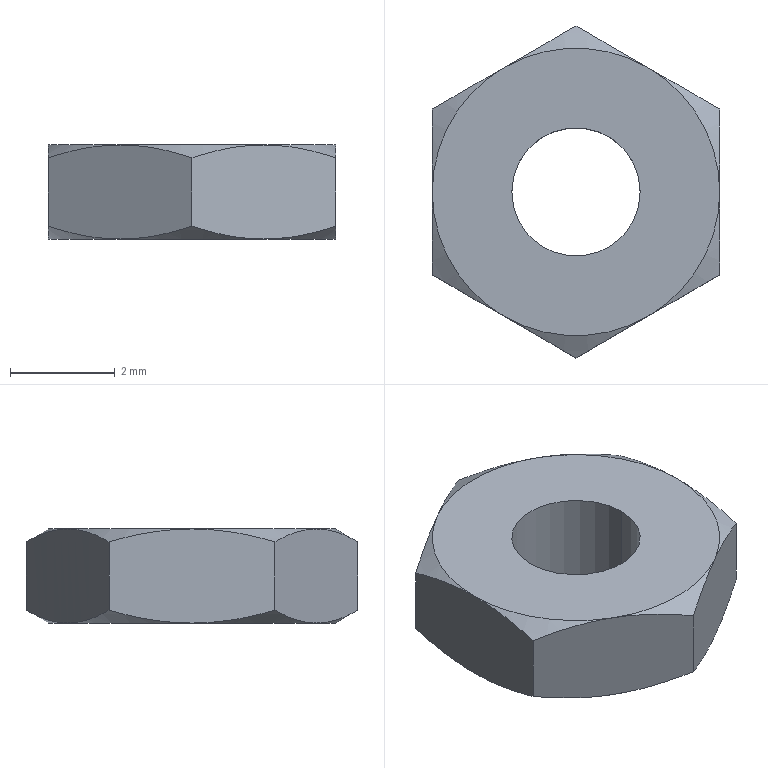Part | SolidWorks | features MBimport 1 | 1 solid | 22 faces | box 5.5 x 6.351 x 1.8 mm | volume 38.249 mm3 | cone 12 | plane 8 | cylinder 2 | commonest cylinder face diameters 2.459 x2
STEP:
#1=CARTESIAN_POINT('',(-1.375,2.382,1.8));
#2=VERTEX_POINT('',#1);
#3=CARTESIAN_POINT('',(-2.75,1.588,1.554));
#4=VERTEX_POINT('',#3);
#5=CARTESIAN_POINT('',(-1.375,2.382,1.8));
#6=CARTESIAN_POINT('',(-1.492,2.314,1.8));
#7=CARTESIAN_POINT('',(-1.606,2.248,1.794));
#8=CARTESIAN_POINT('',(-1.779,2.148,1.778));
#9=CARTESIAN_POINT('',(-1.837,2.115,1.771));
#10=CARTESIAN_POINT('',(-1.924,2.065,1.759));
#11=CARTESIAN_POINT('',(-1.953,2.048,1.754));
#12=CARTESIAN_POINT('',(-2.011,2.014,1.744));
#13=CARTESIAN_POINT('',(-2.043,1.996,1.739));
#14=CARTESIAN_POINT('',(-2.293,1.852,1.692));
#15=CARTESIAN_POINT('',(-2.516,1.723,1.632));
#16=CARTESIAN_POINT('',(-2.75,1.588,1.554));
#17=B_SPLINE_CURVE_WITH_KNOTS('',3,(#5,#6,#7,#8,#9,#10,#11,#12,#13,#14,#15,#16),.UNSPECIFIED.,.F.,.F.,(4,2,2,2,2,4),(0.,0.25,0.375,0.4375,0.5,1.),.UNSPECIFIED.);
#18=EDGE_CURVE('',#2,#4,#17,.T.);
#19=ORIENTED_EDGE('',*,*,#18,.T.);
#20=CARTESIAN_POINT('',(-2.75,0.,1.8));
#21=VERTEX_POINT('',#20);
#22=CARTESIAN_POINT('',(-2.75,1.588,1.554));
#23=CARTESIAN_POINT('',(-2.75,1.453,1.593));
#24=CARTESIAN_POINT('',(-2.75,1.321,1.628));
#25=CARTESIAN_POINT('',(-2.75,1.127,1.672));
#26=CARTESIAN_POINT('',(-2.75,1.062,1.686));
#27=CARTESIAN_POINT('',(-2.75,0.9659,1.705));
#28=CARTESIAN_POINT('',(-2.75,0.9178,1.714));
#29=CARTESIAN_POINT('',(-2.75,0.8699,1.722));
#30=CARTESIAN_POINT('',(-2.75,0.8379,1.728));
#31=CARTESIAN_POINT('',(-2.75,0.8231,1.73));
#32=CARTESIAN_POINT('',(-2.75,0.5318,1.778));
#33=CARTESIAN_POINT('',(-2.75,0.2702,1.8));
#34=CARTESIAN_POINT('',(-2.75,0.,1.8));
#35=B_SPLINE_CURVE_WITH_KNOTS('',3,(#22,#23,#24,#25,#26,#27,#28,#29,#30,#31,#32,#33,#34),.UNSPECIFIED.,.F.,.F.,(4,2,2,1,2,2,4),(0.,0.25,0.375,0.4375,0.4688,0.5,1.),.UNSPECIFIED.);
#36=EDGE_CURVE('',#4,#21,#35,.T.);
#37=ORIENTED_EDGE('',*,*,#36,.T.);
#38=CARTESIAN_POINT('',(0.,0.,1.8));
#39=DIRECTION('',(0.,0.,-1.));
#40=DIRECTION('',(-1.,0.,0.));
#41=AXIS2_PLACEMENT_3D('',#38,#39,#40);
#42=CIRCLE('',#41,2.75);
#43=EDGE_CURVE('',#21,#2,#42,.T.);
#44=ORIENTED_EDGE('',*,*,#43,.T.);
#45=EDGE_LOOP('',(#19,#37,#44));
#46=FACE_OUTER_BOUND('',#45,.T.);
#47=CARTESIAN_POINT('',(0.,0.,1.8));
#48=DIRECTION('',(0.,0.,-1.));
#49=DIRECTION('',(1.,0.,0.));
#50=AXIS2_PLACEMENT_3D('',#47,#48,#49);
#51=CONICAL_SURFACE('',#50,2.75,1.047);
#52=ADVANCED_FACE('',(#46),#51,.T.);
#53=CARTESIAN_POINT('',(1.375,2.382,1.8));
#54=VERTEX_POINT('',#53);
#55=CARTESIAN_POINT('',(0.,3.175,1.554));
#56=VERTEX_POINT('',#55);
#57=CARTESIAN_POINT('',(1.375,2.382,1.8));
#58=CARTESIAN_POINT('',(1.258,2.449,1.8));
#59=CARTESIAN_POINT('',(1.144,2.515,1.794));
#60=CARTESIAN_POINT('',(0.971,2.615,1.778));
#61=CARTESIAN_POINT('',(0.9133,2.648,1.771));
#62=CARTESIAN_POINT('',(0.8262,2.698,1.759));
#63=CARTESIAN_POINT('',(0.7971,2.715,1.754));
#64=CARTESIAN_POINT('',(0.7385,2.749,1.744));
#65=CARTESIAN_POINT('',(0.7073,2.767,1.739));
#66=CARTESIAN_POINT('',(0.4575,2.911,1.692));
#67=CARTESIAN_POINT('',(0.2341,3.04,1.632));
#68=CARTESIAN_POINT('',(0.,3.175,1.554));
#69=B_SPLINE_CURVE_WITH_KNOTS('',3,(#57,#58,#59,#60,#61,#62,#63,#64,#65,#66,#67,#68),.UNSPECIFIED.,.F.,.F.,(4,2,2,2,2,4),(0.,0.25,0.375,0.4375,0.5,1.),.UNSPECIFIED.);
#70=EDGE_CURVE('',#54,#56,#69,.T.);
#71=ORIENTED_EDGE('',*,*,#70,.T.);
#72=CARTESIAN_POINT('',(0.,3.175,1.554));
#73=CARTESIAN_POINT('',(-0.1171,3.108,1.593));
#74=CARTESIAN_POINT('',(-0.2316,3.042,1.628));
#75=CARTESIAN_POINT('',(-0.4011,2.944,1.673));
#76=CARTESIAN_POINT('',(-0.4573,2.912,1.687));
#77=CARTESIAN_POINT('',(-0.5412,2.863,1.706));
#78=CARTESIAN_POINT('',(-0.5691,2.847,1.712));
#79=CARTESIAN_POINT('',(-0.6249,2.815,1.723));
#80=CARTESIAN_POINT('',(-0.651,2.8,1.728));
#81=CARTESIAN_POINT('',(-0.9173,2.646,1.778));
#82=CARTESIAN_POINT('',(-1.143,2.516,1.8));
#83=CARTESIAN_POINT('',(-1.375,2.382,1.8));
#84=B_SPLINE_CURVE_WITH_KNOTS('',3,(#72,#73,#74,#75,#76,#77,#78,#79,#80,#81,#82,#83),.UNSPECIFIED.,.F.,.F.,(4,2,2,2,2,4),(0.,0.25,0.375,0.4375,0.5,1.),.UNSPECIFIED.);
#85=EDGE_CURVE('',#56,#2,#84,.T.);
#86=ORIENTED_EDGE('',*,*,#85,.T.);
#87=CARTESIAN_POINT('',(0.,0.,1.8));
#88=DIRECTION('',(0.,0.,-1.));
#89=DIRECTION('',(-1.,0.,0.));
#90=AXIS2_PLACEMENT_3D('',#87,#88,#89);
#91=CIRCLE('',#90,2.75);
#92=EDGE_CURVE('',#2,#54,#91,.T.);
#93=ORIENTED_EDGE('',*,*,#92,.T.);
#94=EDGE_LOOP('',(#71,#86,#93));
#95=FACE_OUTER_BOUND('',#94,.T.);
#96=CARTESIAN_POINT('',(0.,0.,1.8));
#97=DIRECTION('',(0.,0.,-1.));
#98=DIRECTION('',(1.,0.,0.));
#99=AXIS2_PLACEMENT_3D('',#96,#97,#98);
#100=CONICAL_SURFACE('',#99,2.75,1.047);
#101=ADVANCED_FACE('',(#95),#100,.T.);
#102=CARTESIAN_POINT('',(2.75,1.588,1.554));
#103=VERTEX_POINT('',#102);
#104=CARTESIAN_POINT('',(2.75,1.588,1.554));
#105=CARTESIAN_POINT('',(2.633,1.655,1.593));
#106=CARTESIAN_POINT('',(2.518,1.721,1.628));
#107=CARTESIAN_POINT('',(2.349,1.819,1.673));
#108=CARTESIAN_POINT('',(2.293,1.852,1.687));
#109=CARTESIAN_POINT('',(2.209,1.9,1.706));
#110=CARTESIAN_POINT('',(2.181,1.916,1.712));
#111=CARTESIAN_POINT('',(2.125,1.949,1.723));
#112=CARTESIAN_POINT('',(2.099,1.964,1.728));
#113=CARTESIAN_POINT('',(1.833,2.117,1.778));
#114=CARTESIAN_POINT('',(1.607,2.247,1.8));
#115=CARTESIAN_POINT('',(1.375,2.382,1.8));
#116=B_SPLINE_CURVE_WITH_KNOTS('',3,(#104,#105,#106,#107,#108,#109,#110,#111,#112,#113,#114,#115),.UNSPECIFIED.,.F.,.F.,(4,2,2,2,2,4),(0.,0.25,0.375,0.4375,0.5,1.),.UNSPECIFIED.);
#117=EDGE_CURVE('',#103,#54,#116,.T.);
#118=ORIENTED_EDGE('',*,*,#117,.T.);
#119=CARTESIAN_POINT('',(2.75,0.,1.8));
#120=VERTEX_POINT('',#119);
#121=CARTESIAN_POINT('',(0.,0.,1.8));
#122=DIRECTION('',(0.,0.,1.));
#123=DIRECTION('',(1.,0.,0.));
#124=AXIS2_PLACEMENT_3D('',#121,#122,#123);
#125=CIRCLE('',#124,2.75);
#126=EDGE_CURVE('',#120,#54,#125,.T.);
#127=ORIENTED_EDGE('',*,*,#126,.F.);
#128=CARTESIAN_POINT('',(2.75,0.,1.8));
#129=CARTESIAN_POINT('',(2.75,0.1351,1.8));
#130=CARTESIAN_POINT('',(2.75,0.268,1.794));
#131=CARTESIAN_POINT('',(2.75,0.4681,1.778));
#132=CARTESIAN_POINT('',(2.75,0.535,1.771));
#133=CARTESIAN_POINT('',(2.75,0.6359,1.758));
#134=CARTESIAN_POINT('',(2.75,0.6866,1.751));
#135=CARTESIAN_POINT('',(2.75,0.7376,1.744));
#136=CARTESIAN_POINT('',(2.75,0.7717,1.739));
#137=CARTESIAN_POINT('',(2.75,0.79,1.736));
#138=CARTESIAN_POINT('',(2.75,1.061,1.692));
#139=CARTESIAN_POINT('',(2.75,1.318,1.632));
#140=CARTESIAN_POINT('',(2.75,1.588,1.554));
#141=B_SPLINE_CURVE_WITH_KNOTS('',3,(#128,#129,#130,#131,#132,#133,#134,#135,#136,#137,#138,#139,#140),.UNSPECIFIED.,.F.,.F.,(4,2,2,1,2,2,4),(0.,0.25,0.375,0.4375,0.4687,0.5,1.),.UNSPECIFIED.);
#142=EDGE_CURVE('',#120,#103,#141,.T.);
#143=ORIENTED_EDGE('',*,*,#142,.T.);
#144=EDGE_LOOP('',(#118,#127,#143));
#145=FACE_OUTER_BOUND('',#144,.T.);
#146=CARTESIAN_POINT('',(0.,0.,1.8));
#147=DIRECTION('',(0.,0.,-1.));
#148=DIRECTION('',(1.,0.,0.));
#149=AXIS2_PLACEMENT_3D('',#146,#147,#148);
#150=CONICAL_SURFACE('',#149,2.75,1.047);
#151=ADVANCED_FACE('',(#145),#150,.T.);
#152=CARTESIAN_POINT('',(1.375,-2.382,1.8));
#153=VERTEX_POINT('',#152);
#154=CARTESIAN_POINT('',(2.75,-1.588,1.554));
#155=VERTEX_POINT('',#154);
#156=CARTESIAN_POINT('',(1.375,-2.382,1.8));
#157=CARTESIAN_POINT('',(1.492,-2.314,1.8));
#158=CARTESIAN_POINT('',(1.606,-2.248,1.794));
#159=CARTESIAN_POINT('',(1.779,-2.148,1.778));
#160=CARTESIAN_POINT('',(1.837,-2.115,1.771));
#161=CARTESIAN_POINT('',(1.924,-2.065,1.759));
#162=CARTESIAN_POINT('',(1.953,-2.048,1.754));
#163=CARTESIAN_POINT('',(2.011,-2.014,1.744));
#164=CARTESIAN_POINT('',(2.043,-1.996,1.739));
#165=CARTESIAN_POINT('',(2.293,-1.852,1.692));
#166=CARTESIAN_POINT('',(2.516,-1.723,1.632));
#167=CARTESIAN_POINT('',(2.75,-1.588,1.554));
#168=B_SPLINE_CURVE_WITH_KNOTS('',3,(#156,#157,#158,#159,#160,#161,#162,#163,#164,#165,#166,#167),.UNSPECIFIED.,.F.,.F.,(4,2,2,2,2,4),(0.,0.25,0.375,0.4375,0.5,1.),.UNSPECIFIED.);
#169=EDGE_CURVE('',#153,#155,#168,.T.);
#170=ORIENTED_EDGE('',*,*,#169,.T.);
#171=CARTESIAN_POINT('',(2.75,-1.588,1.554));
#172=CARTESIAN_POINT('',(2.75,-1.452,1.594));
#173=CARTESIAN_POINT('',(2.75,-1.319,1.628));
#174=CARTESIAN_POINT('',(2.75,-1.123,1.673));
#175=CARTESIAN_POINT('',(2.75,-1.058,1.687));
#176=CARTESIAN_POINT('',(2.75,-0.9612,1.706));
#177=CARTESIAN_POINT('',(2.75,-0.9289,1.712));
#178=CARTESIAN_POINT('',(2.75,-0.8644,1.724));
#179=CARTESIAN_POINT('',(2.75,-0.834,1.729));
#180=CARTESIAN_POINT('',(2.75,-0.5279,1.778));
#181=CARTESIAN_POINT('',(2.75,-0.2682,1.8));
#182=CARTESIAN_POINT('',(2.75,0.,1.8));
#183=B_SPLINE_CURVE_WITH_KNOTS('',3,(#171,#172,#173,#174,#175,#176,#177,#178,#179,#180,#181,#182),.UNSPECIFIED.,.F.,.F.,(4,2,2,2,2,4),(0.,0.25,0.375,0.4375,0.5,1.),.UNSPECIFIED.);
#184=EDGE_CURVE('',#155,#120,#183,.T.);
#185=ORIENTED_EDGE('',*,*,#184,.T.);
#186=CARTESIAN_POINT('',(0.,0.,1.8));
#187=DIRECTION('',(0.,0.,-1.));
#188=DIRECTION('',(-1.,0.,0.));
#189=AXIS2_PLACEMENT_3D('',#186,#187,#188);
#190=CIRCLE('',#189,2.75);
#191=EDGE_CURVE('',#120,#153,#190,.T.);
#192=ORIENTED_EDGE('',*,*,#191,.T.);
#193=EDGE_LOOP('',(#170,#185,#192));
#194=FACE_OUTER_BOUND('',#193,.T.);
#195=CARTESIAN_POINT('',(0.,0.,1.8));
#196=DIRECTION('',(0.,0.,-1.));
#197=DIRECTION('',(1.,0.,0.));
#198=AXIS2_PLACEMENT_3D('',#195,#196,#197);
#199=CONICAL_SURFACE('',#198,2.75,1.047);
#200=ADVANCED_FACE('',(#194),#199,.T.);
#201=CARTESIAN_POINT('',(-1.375,-2.382,1.8));
#202=VERTEX_POINT('',#201);
#203=CARTESIAN_POINT('',(0.,-3.175,1.554));
#204=VERTEX_POINT('',#203);
#205=CARTESIAN_POINT('',(-1.375,-2.382,1.8));
#206=CARTESIAN_POINT('',(-1.258,-2.449,1.8));
#207=CARTESIAN_POINT('',(-1.144,-2.515,1.794));
#208=CARTESIAN_POINT('',(-0.971,-2.615,1.778));
#209=CARTESIAN_POINT('',(-0.9133,-2.648,1.771));
#210=CARTESIAN_POINT('',(-0.8262,-2.698,1.759));
#211=CARTESIAN_POINT('',(-0.7971,-2.715,1.754));
#212=CARTESIAN_POINT('',(-0.7385,-2.749,1.744));
#213=CARTESIAN_POINT('',(-0.7073,-2.767,1.739));
#214=CARTESIAN_POINT('',(-0.4575,-2.911,1.692));
#215=CARTESIAN_POINT('',(-0.2341,-3.04,1.632));
#216=CARTESIAN_POINT('',(0.,-3.175,1.554));
#217=B_SPLINE_CURVE_WITH_KNOTS('',3,(#205,#206,#207,#208,#209,#210,#211,#212,#213,#214,#215,#216),.UNSPECIFIED.,.F.,.F.,(4,2,2,2,2,4),(0.,0.25,0.375,0.4375,0.5,1.),.UNSPECIFIED.);
#218=EDGE_CURVE('',#202,#204,#217,.T.);
#219=ORIENTED_EDGE('',*,*,#218,.T.);
#220=CARTESIAN_POINT('',(0.,-3.175,1.554));
#221=CARTESIAN_POINT('',(0.1171,-3.108,1.593));
#222=CARTESIAN_POINT('',(0.2316,-3.042,1.628));
#223=CARTESIAN_POINT('',(0.4011,-2.944,1.673));
#224=CARTESIAN_POINT('',(0.4573,-2.912,1.687));
#225=CARTESIAN_POINT('',(0.5412,-2.863,1.706));
#226=CARTESIAN_POINT('',(0.5691,-2.847,1.712));
#227=CARTESIAN_POINT('',(0.6249,-2.815,1.723));
#228=CARTESIAN_POINT('',(0.651,-2.8,1.728));
#229=CARTESIAN_POINT('',(0.9173,-2.646,1.778));
#230=CARTESIAN_POINT('',(1.143,-2.516,1.8));
#231=CARTESIAN_POINT('',(1.375,-2.382,1.8));
#232=B_SPLINE_CURVE_WITH_KNOTS('',3,(#220,#221,#222,#223,#224,#225,#226,#227,#228,#229,#230,#231),.UNSPECIFIED.,.F.,.F.,(4,2,2,2,2,4),(0.,0.25,0.375,0.4375,0.5,1.),.UNSPECIFIED.);
#233=EDGE_CURVE('',#204,#153,#232,.T.);
#234=ORIENTED_EDGE('',*,*,#233,.T.);
#235=CARTESIAN_POINT('',(0.,0.,1.8));
#236=DIRECTION('',(0.,0.,-1.));
#237=DIRECTION('',(-1.,0.,0.));
#238=AXIS2_PLACEMENT_3D('',#235,#236,#237);
#239=CIRCLE('',#238,2.75);
#240=EDGE_CURVE('',#153,#202,#239,.T.);
#241=ORIENTED_EDGE('',*,*,#240,.T.);
#242=EDGE_LOOP('',(#219,#234,#241));
#243=FACE_OUTER_BOUND('',#242,.T.);
#244=CARTESIAN_POINT('',(0.,0.,1.8));
#245=DIRECTION('',(0.,0.,-1.));
#246=DIRECTION('',(1.,0.,0.));
#247=AXIS2_PLACEMENT_3D('',#244,#245,#246);
#248=CONICAL_SURFACE('',#247,2.75,1.047);
#249=ADVANCED_FACE('',(#243),#248,.T.);
#250=CARTESIAN_POINT('',(-2.75,-1.588,1.554));
#251=VERTEX_POINT('',#250);
#252=CARTESIAN_POINT('',(-2.75,0.,1.8));
#253=CARTESIAN_POINT('',(-2.75,-0.1341,1.8));
#254=CARTESIAN_POINT('',(-2.75,-0.266,1.795));
#255=CARTESIAN_POINT('',(-2.75,-0.4647,1.778));
#256=CARTESIAN_POINT('',(-2.75,-0.5311,1.771));
#257=CARTESIAN_POINT('',(-2.75,-0.6313,1.759));
#258=CARTESIAN_POINT('',(-2.75,-0.6648,1.754));
#259=CARTESIAN_POINT('',(-2.75,-0.7322,1.745));
#260=CARTESIAN_POINT('',(-2.75,-0.7678,1.739));
#261=CARTESIAN_POINT('',(-2.75,-1.057,1.693));
#262=CARTESIAN_POINT('',(-2.75,-1.316,1.633));
#263=CARTESIAN_POINT('',(-2.75,-1.588,1.554));
#264=B_SPLINE_CURVE_WITH_KNOTS('',3,(#252,#253,#254,#255,#256,#257,#258,#259,#260,#261,#262,#263),.UNSPECIFIED.,.F.,.F.,(4,2,2,2,2,4),(0.,0.25,0.375,0.4375,0.5,1.),.UNSPECIFIED.);
#265=EDGE_CURVE('',#21,#251,#264,.T.);
#266=ORIENTED_EDGE('',*,*,#265,.T.);
#267=CARTESIAN_POINT('',(-2.75,-1.588,1.554));
#268=CARTESIAN_POINT('',(-2.633,-1.655,1.593));
#269=CARTESIAN_POINT('',(-2.518,-1.721,1.628));
#270=CARTESIAN_POINT('',(-2.349,-1.819,1.673));
#271=CARTESIAN_POINT('',(-2.293,-1.852,1.687));
#272=CARTESIAN_POINT('',(-2.209,-1.9,1.706));
#273=CARTESIAN_POINT('',(-2.181,-1.916,1.712));
#274=CARTESIAN_POINT('',(-2.125,-1.949,1.723));
#275=CARTESIAN_POINT('',(-2.099,-1.964,1.728));
#276=CARTESIAN_POINT('',(-1.833,-2.117,1.778));
#277=CARTESIAN_POINT('',(-1.607,-2.247,1.8));
#278=CARTESIAN_POINT('',(-1.375,-2.382,1.8));
#279=B_SPLINE_CURVE_WITH_KNOTS('',3,(#267,#268,#269,#270,#271,#272,#273,#274,#275,#276,#277,#278),.UNSPECIFIED.,.F.,.F.,(4,2,2,2,2,4),(0.,0.25,0.375,0.4375,0.5,1.),.UNSPECIFIED.);
#280=EDGE_CURVE('',#251,#202,#279,.T.);
#281=ORIENTED_EDGE('',*,*,#280,.T.);
#282=CARTESIAN_POINT('',(0.,0.,1.8));
#283=DIRECTION('',(0.,0.,-1.));
#284=DIRECTION('',(-1.,0.,0.));
#285=AXIS2_PLACEMENT_3D('',#282,#283,#284);
#286=CIRCLE('',#285,2.75);
#287=EDGE_CURVE('',#202,#21,#286,.T.);
#288=ORIENTED_EDGE('',*,*,#287,.T.);
#289=EDGE_LOOP('',(#266,#281,#288));
#290=FACE_OUTER_BOUND('',#289,.T.);
#291=CARTESIAN_POINT('',(0.,0.,1.8));
#292=DIRECTION('',(0.,0.,-1.));
#293=DIRECTION('',(1.,0.,0.));
#294=AXIS2_PLACEMENT_3D('',#291,#292,#293);
#295=CONICAL_SURFACE('',#294,2.75,1.047);
#296=ADVANCED_FACE('',(#290),#295,.T.);
#297=CARTESIAN_POINT('',(-1.375,2.382,0.));
#298=VERTEX_POINT('',#297);
#299=CARTESIAN_POINT('',(0.,3.175,0.2456));
#300=VERTEX_POINT('',#299);
#301=CARTESIAN_POINT('',(-1.375,2.382,0.));
#302=CARTESIAN_POINT('',(-1.258,2.449,0.));
#303=CARTESIAN_POINT('',(-1.144,2.515,0.005525));
#304=CARTESIAN_POINT('',(-0.971,2.615,0.0221));
#305=CARTESIAN_POINT('',(-0.9133,2.648,0.02901));
#306=CARTESIAN_POINT('',(-0.8262,2.698,0.04144));
#307=CARTESIAN_POINT('',(-0.7971,2.715,0.04593));
#308=CARTESIAN_POINT('',(-0.7385,2.749,0.0556));
#309=CARTESIAN_POINT('',(-0.7073,2.767,0.06112));
#310=CARTESIAN_POINT('',(-0.4575,2.911,0.1078));
#311=CARTESIAN_POINT('',(-0.2341,3.04,0.1676));
#312=CARTESIAN_POINT('',(0.,3.175,0.2456));
#313=B_SPLINE_CURVE_WITH_KNOTS('',3,(#301,#302,#303,#304,#305,#306,#307,#308,#309,#310,#311,#312),.UNSPECIFIED.,.F.,.F.,(4,2,2,2,2,4),(0.,0.25,0.375,0.4375,0.5,1.),.UNSPECIFIED.);
#314=EDGE_CURVE('',#298,#300,#313,.T.);
#315=ORIENTED_EDGE('',*,*,#314,.T.);
#316=CARTESIAN_POINT('',(1.375,2.382,0.));
#317=VERTEX_POINT('',#316);
#318=CARTESIAN_POINT('',(0.,3.175,0.2456));
#319=CARTESIAN_POINT('',(0.1171,3.108,0.2066));
#320=CARTESIAN_POINT('',(0.2316,3.042,0.1721));
#321=CARTESIAN_POINT('',(0.4011,2.944,0.1273));
#322=CARTESIAN_POINT('',(0.4573,2.912,0.1135));
#323=CARTESIAN_POINT('',(0.5412,2.863,0.09449));
#324=CARTESIAN_POINT('',(0.5691,2.847,0.08844));
#325=CARTESIAN_POINT('',(0.6249,2.815,0.07691));
#326=CARTESIAN_POINT('',(0.651,2.8,0.07176));
#327=CARTESIAN_POINT('',(0.9173,2.646,0.02208));
#328=CARTESIAN_POINT('',(1.143,2.516,0.));
#329=CARTESIAN_POINT('',(1.375,2.382,0.));
#330=B_SPLINE_CURVE_WITH_KNOTS('',3,(#318,#319,#320,#321,#322,#323,#324,#325,#326,#327,#328,#329),.UNSPECIFIED.,.F.,.F.,(4,2,2,2,2,4),(0.,0.25,0.375,0.4375,0.5,1.),.UNSPECIFIED.);
#331=EDGE_CURVE('',#300,#317,#330,.T.);
#332=ORIENTED_EDGE('',*,*,#331,.T.);
#333=CARTESIAN_POINT('',(0.,0.,0.));
#334=DIRECTION('',(0.,0.,-1.));
#335=DIRECTION('',(-1.,0.,0.));
#336=AXIS2_PLACEMENT_3D('',#333,#334,#335);
#337=CIRCLE('',#336,2.75);
#338=EDGE_CURVE('',#298,#317,#337,.T.);
#339=ORIENTED_EDGE('',*,*,#338,.F.);
#340=EDGE_LOOP('',(#315,#332,#339));
#341=FACE_OUTER_BOUND('',#340,.T.);
#342=CARTESIAN_POINT('',(0.,0.,0.));
#343=DIRECTION('',(0.,0.,1.));
#344=DIRECTION('',(-1.,0.,0.));
#345=AXIS2_PLACEMENT_3D('',#342,#343,#344);
#346=CONICAL_SURFACE('',#345,2.75,1.047);
#347=ADVANCED_FACE('',(#341),#346,.T.);
#348=CARTESIAN_POINT('',(-2.75,0.,0.));
#349=VERTEX_POINT('',#348);
#350=CARTESIAN_POINT('',(-2.75,1.588,0.2456));
#351=VERTEX_POINT('',#350);
#352=CARTESIAN_POINT('',(-2.75,0.,0.));
#353=CARTESIAN_POINT('',(-2.75,0.1351,0.));
#354=CARTESIAN_POINT('',(-2.75,0.268,0.005565));
#355=CARTESIAN_POINT('',(-2.75,0.4681,0.02226));
#356=CARTESIAN_POINT('',(-2.75,0.535,0.02922));
#357=CARTESIAN_POINT('',(-2.75,0.6359,0.04174));
#358=CARTESIAN_POINT('',(-2.75,0.6866,0.04852));
#359=CARTESIAN_POINT('',(-2.75,0.7376,0.05608));
#360=CARTESIAN_POINT('',(-2.75,0.7717,0.0613));
#361=CARTESIAN_POINT('',(-2.75,0.79,0.06419));
#362=CARTESIAN_POINT('',(-2.75,1.061,0.1083));
#363=CARTESIAN_POINT('',(-2.75,1.318,0.1679));
#364=CARTESIAN_POINT('',(-2.75,1.588,0.2456));
#365=B_SPLINE_CURVE_WITH_KNOTS('',3,(#352,#353,#354,#355,#356,#357,#358,#359,#360,#361,#362,#363,#364),.UNSPECIFIED.,.F.,.F.,(4,2,2,1,2,2,4),(0.,0.25,0.375,0.4375,0.4687,0.5,1.),.UNSPECIFIED.);
#366=EDGE_CURVE('',#349,#351,#365,.T.);
#367=ORIENTED_EDGE('',*,*,#366,.T.);
#368=CARTESIAN_POINT('',(-2.75,1.588,0.2456));
#369=CARTESIAN_POINT('',(-2.633,1.655,0.2066));
#370=CARTESIAN_POINT('',(-2.518,1.721,0.1721));
#371=CARTESIAN_POINT('',(-2.349,1.819,0.1273));
#372=CARTESIAN_POINT('',(-2.293,1.852,0.1135));
#373=CARTESIAN_POINT('',(-2.209,1.9,0.09449));
#374=CARTESIAN_POINT('',(-2.181,1.916,0.08844));
#375=CARTESIAN_POINT('',(-2.125,1.949,0.07691));
#376=CARTESIAN_POINT('',(-2.099,1.964,0.07176));
#377=CARTESIAN_POINT('',(-1.833,2.117,0.02208));
#378=CARTESIAN_POINT('',(-1.607,2.247,0.));
#379=CARTESIAN_POINT('',(-1.375,2.382,0.));
#380=B_SPLINE_CURVE_WITH_KNOTS('',3,(#368,#369,#370,#371,#372,#373,#374,#375,#376,#377,#378,#379),.UNSPECIFIED.,.F.,.F.,(4,2,2,2,2,4),(0.,0.25,0.375,0.4375,0.5,1.),.UNSPECIFIED.);
#381=EDGE_CURVE('',#351,#298,#380,.T.);
#382=ORIENTED_EDGE('',*,*,#381,.T.);
#383=CARTESIAN_POINT('',(0.,0.,0.));
#384=DIRECTION('',(0.,0.,-1.));
#385=DIRECTION('',(-1.,0.,0.));
#386=AXIS2_PLACEMENT_3D('',#383,#384,#385);
#387=CIRCLE('',#386,2.75);
#388=EDGE_CURVE('',#349,#298,#387,.T.);
#389=ORIENTED_EDGE('',*,*,#388,.F.);
#390=EDGE_LOOP('',(#367,#382,#389));
#391=FACE_OUTER_BOUND('',#390,.T.);
#392=CARTESIAN_POINT('',(0.,0.,0.));
#393=DIRECTION('',(0.,0.,1.));
#394=DIRECTION('',(-1.,0.,0.));
#395=AXIS2_PLACEMENT_3D('',#392,#393,#394);
#396=CONICAL_SURFACE('',#395,2.75,1.047);
#397=ADVANCED_FACE('',(#391),#396,.T.);
#398=CARTESIAN_POINT('',(-2.75,-1.588,0.2456));
#399=VERTEX_POINT('',#398);
#400=CARTESIAN_POINT('',(-2.75,-1.588,0.2456));
#401=CARTESIAN_POINT('',(-2.75,-1.452,0.2064));
#402=CARTESIAN_POINT('',(-2.75,-1.319,0.1719));
#403=CARTESIAN_POINT('',(-2.75,-1.123,0.1269));
#404=CARTESIAN_POINT('',(-2.75,-1.058,0.1131));
#405=CARTESIAN_POINT('',(-2.75,-0.9612,0.09408));
#406=CARTESIAN_POINT('',(-2.75,-0.9289,0.08802));
#407=CARTESIAN_POINT('',(-2.75,-0.8644,0.07649));
#408=CARTESIAN_POINT('',(-2.75,-0.834,0.07131));
#409=CARTESIAN_POINT('',(-2.75,-0.5279,0.02194));
#410=CARTESIAN_POINT('',(-2.75,-0.2682,0.));
#411=CARTESIAN_POINT('',(-2.75,0.,0.));
#412=B_SPLINE_CURVE_WITH_KNOTS('',3,(#400,#401,#402,#403,#404,#405,#406,#407,#408,#409,#410,#411),.UNSPECIFIED.,.F.,.F.,(4,2,2,2,2,4),(0.,0.25,0.375,0.4375,0.5,1.),.UNSPECIFIED.);
#413=EDGE_CURVE('',#399,#349,#412,.T.);
#414=ORIENTED_EDGE('',*,*,#413,.T.);
#415=CARTESIAN_POINT('',(-1.375,-2.382,0.));
#416=VERTEX_POINT('',#415);
#417=CARTESIAN_POINT('',(0.,0.,0.));
#418=DIRECTION('',(0.,0.,-1.));
#419=DIRECTION('',(-1.,0.,0.));
#420=AXIS2_PLACEMENT_3D('',#417,#418,#419);
#421=CIRCLE('',#420,2.75);
#422=EDGE_CURVE('',#416,#349,#421,.T.);
#423=ORIENTED_EDGE('',*,*,#422,.F.);
#424=CARTESIAN_POINT('',(-1.375,-2.382,0.));
#425=CARTESIAN_POINT('',(-1.492,-2.314,0.));
#426=CARTESIAN_POINT('',(-1.606,-2.248,0.005525));
#427=CARTESIAN_POINT('',(-1.779,-2.148,0.0221));
#428=CARTESIAN_POINT('',(-1.837,-2.115,0.02901));
#429=CARTESIAN_POINT('',(-1.924,-2.065,0.04144));
#430=CARTESIAN_POINT('',(-1.953,-2.048,0.04593));
#431=CARTESIAN_POINT('',(-2.011,-2.014,0.0556));
#432=CARTESIAN_POINT('',(-2.043,-1.996,0.06112));
#433=CARTESIAN_POINT('',(-2.293,-1.852,0.1078));
#434=CARTESIAN_POINT('',(-2.516,-1.723,0.1676));
#435=CARTESIAN_POINT('',(-2.75,-1.588,0.2456));
#436=B_SPLINE_CURVE_WITH_KNOTS('',3,(#424,#425,#426,#427,#428,#429,#430,#431,#432,#433,#434,#435),.UNSPECIFIED.,.F.,.F.,(4,2,2,2,2,4),(0.,0.25,0.375,0.4375,0.5,1.),.UNSPECIFIED.);
#437=EDGE_CURVE('',#416,#399,#436,.T.);
#438=ORIENTED_EDGE('',*,*,#437,.T.);
#439=EDGE_LOOP('',(#414,#423,#438));
#440=FACE_OUTER_BOUND('',#439,.T.);
#441=CARTESIAN_POINT('',(0.,0.,0.));
#442=DIRECTION('',(0.,0.,1.));
#443=DIRECTION('',(-1.,0.,0.));
#444=AXIS2_PLACEMENT_3D('',#441,#442,#443);
#445=CONICAL_SURFACE('',#444,2.75,1.047);
#446=ADVANCED_FACE('',(#440),#445,.T.);
#447=CARTESIAN_POINT('',(0.,-3.175,0.2456));
#448=VERTEX_POINT('',#447);
#449=CARTESIAN_POINT('',(0.,-3.175,0.2456));
#450=CARTESIAN_POINT('',(-0.1171,-3.108,0.2066));
#451=CARTESIAN_POINT('',(-0.2316,-3.042,0.1721));
#452=CARTESIAN_POINT('',(-0.4011,-2.944,0.1273));
#453=CARTESIAN_POINT('',(-0.4573,-2.912,0.1135));
#454=CARTESIAN_POINT('',(-0.5412,-2.863,0.09449));
#455=CARTESIAN_POINT('',(-0.5691,-2.847,0.08844));
#456=CARTESIAN_POINT('',(-0.6249,-2.815,0.07691));
#457=CARTESIAN_POINT('',(-0.651,-2.8,0.07176));
#458=CARTESIAN_POINT('',(-0.9173,-2.646,0.02208));
#459=CARTESIAN_POINT('',(-1.143,-2.516,0.));
#460=CARTESIAN_POINT('',(-1.375,-2.382,0.));
#461=B_SPLINE_CURVE_WITH_KNOTS('',3,(#449,#450,#451,#452,#453,#454,#455,#456,#457,#458,#459,#460),.UNSPECIFIED.,.F.,.F.,(4,2,2,2,2,4),(0.,0.25,0.375,0.4375,0.5,1.),.UNSPECIFIED.);
#462=EDGE_CURVE('',#448,#416,#461,.T.);
#463=ORIENTED_EDGE('',*,*,#462,.T.);
#464=CARTESIAN_POINT('',(1.375,-2.382,0.));
#465=VERTEX_POINT('',#464);
#466=CARTESIAN_POINT('',(0.,0.,0.));
#467=DIRECTION('',(0.,0.,-1.));
#468=DIRECTION('',(-1.,0.,0.));
#469=AXIS2_PLACEMENT_3D('',#466,#467,#468);
#470=CIRCLE('',#469,2.75);
#471=EDGE_CURVE('',#465,#416,#470,.T.);
#472=ORIENTED_EDGE('',*,*,#471,.F.);
#473=CARTESIAN_POINT('',(1.375,-2.382,0.));
#474=CARTESIAN_POINT('',(1.258,-2.449,0.));
#475=CARTESIAN_POINT('',(1.144,-2.515,0.005525));
#476=CARTESIAN_POINT('',(0.971,-2.615,0.0221));
#477=CARTESIAN_POINT('',(0.9133,-2.648,0.02901));
#478=CARTESIAN_POINT('',(0.8262,-2.698,0.04144));
#479=CARTESIAN_POINT('',(0.7971,-2.715,0.04593));
#480=CARTESIAN_POINT('',(0.7385,-2.749,0.0556));
#481=CARTESIAN_POINT('',(0.7073,-2.767,0.06112));
#482=CARTESIAN_POINT('',(0.4575,-2.911,0.1078));
#483=CARTESIAN_POINT('',(0.2341,-3.04,0.1676));
#484=CARTESIAN_POINT('',(0.,-3.175,0.2456));
#485=B_SPLINE_CURVE_WITH_KNOTS('',3,(#473,#474,#475,#476,#477,#478,#479,#480,#481,#482,#483,#484),.UNSPECIFIED.,.F.,.F.,(4,2,2,2,2,4),(0.,0.25,0.375,0.4375,0.5,1.),.UNSPECIFIED.);
#486=EDGE_CURVE('',#465,#448,#485,.T.);
#487=ORIENTED_EDGE('',*,*,#486,.T.);
#488=EDGE_LOOP('',(#463,#472,#487));
#489=FACE_OUTER_BOUND('',#488,.T.);
#490=CARTESIAN_POINT('',(0.,0.,0.));
#491=DIRECTION('',(0.,0.,1.));
#492=DIRECTION('',(-1.,0.,0.));
#493=AXIS2_PLACEMENT_3D('',#490,#491,#492);
#494=CONICAL_SURFACE('',#493,2.75,1.047);
#495=ADVANCED_FACE('',(#489),#494,.T.);
#496=CARTESIAN_POINT('',(2.75,1.588,0.2456));
#497=VERTEX_POINT('',#496);
#498=CARTESIAN_POINT('',(1.375,2.382,0.));
#499=CARTESIAN_POINT('',(1.492,2.314,0.));
#500=CARTESIAN_POINT('',(1.606,2.248,0.005525));
#501=CARTESIAN_POINT('',(1.779,2.148,0.0221));
#502=CARTESIAN_POINT('',(1.837,2.115,0.02901));
#503=CARTESIAN_POINT('',(1.924,2.065,0.04144));
#504=CARTESIAN_POINT('',(1.953,2.048,0.04593));
#505=CARTESIAN_POINT('',(2.011,2.014,0.0556));
#506=CARTESIAN_POINT('',(2.043,1.996,0.06112));
#507=CARTESIAN_POINT('',(2.293,1.852,0.1078));
#508=CARTESIAN_POINT('',(2.516,1.723,0.1676));
#509=CARTESIAN_POINT('',(2.75,1.588,0.2456));
#510=B_SPLINE_CURVE_WITH_KNOTS('',3,(#498,#499,#500,#501,#502,#503,#504,#505,#506,#507,#508,#509),.UNSPECIFIED.,.F.,.F.,(4,2,2,2,2,4),(0.,0.25,0.375,0.4375,0.5,1.),.UNSPECIFIED.);
#511=EDGE_CURVE('',#317,#497,#510,.T.);
#512=ORIENTED_EDGE('',*,*,#511,.T.);
#513=CARTESIAN_POINT('',(2.75,0.,0.));
#514=VERTEX_POINT('',#513);
#515=CARTESIAN_POINT('',(2.75,1.588,0.2456));
#516=CARTESIAN_POINT('',(2.75,1.453,0.2068));
#517=CARTESIAN_POINT('',(2.75,1.321,0.1724));
#518=CARTESIAN_POINT('',(2.75,1.127,0.1277));
#519=CARTESIAN_POINT('',(2.75,1.062,0.1139));
#520=CARTESIAN_POINT('',(2.75,0.9659,0.09498));
#521=CARTESIAN_POINT('',(2.75,0.9178,0.08592));
#522=CARTESIAN_POINT('',(2.75,0.8699,0.07751));
#523=CARTESIAN_POINT('',(2.75,0.8379,0.07204));
#524=CARTESIAN_POINT('',(2.75,0.8231,0.06956));
#525=CARTESIAN_POINT('',(2.75,0.5318,0.02226));
#526=CARTESIAN_POINT('',(2.75,0.2702,0.));
#527=CARTESIAN_POINT('',(2.75,0.,0.));
#528=B_SPLINE_CURVE_WITH_KNOTS('',3,(#515,#516,#517,#518,#519,#520,#521,#522,#523,#524,#525,#526,#527),.UNSPECIFIED.,.F.,.F.,(4,2,2,1,2,2,4),(0.,0.25,0.375,0.4375,0.4688,0.5,1.),.UNSPECIFIED.);
#529=EDGE_CURVE('',#497,#514,#528,.T.);
#530=ORIENTED_EDGE('',*,*,#529,.T.);
#531=CARTESIAN_POINT('',(0.,0.,0.));
#532=DIRECTION('',(0.,0.,-1.));
#533=DIRECTION('',(-1.,0.,0.));
#534=AXIS2_PLACEMENT_3D('',#531,#532,#533);
#535=CIRCLE('',#534,2.75);
#536=EDGE_CURVE('',#317,#514,#535,.T.);
#537=ORIENTED_EDGE('',*,*,#536,.F.);
#538=EDGE_LOOP('',(#512,#530,#537));
#539=FACE_OUTER_BOUND('',#538,.T.);
#540=CARTESIAN_POINT('',(0.,0.,0.));
#541=DIRECTION('',(0.,0.,1.));
#542=DIRECTION('',(-1.,0.,0.));
#543=AXIS2_PLACEMENT_3D('',#540,#541,#542);
#544=CONICAL_SURFACE('',#543,2.75,1.047);
#545=ADVANCED_FACE('',(#539),#544,.T.);
#546=CARTESIAN_POINT('',(2.75,-1.588,0.2456));
#547=VERTEX_POINT('',#546);
#548=CARTESIAN_POINT('',(2.75,-1.588,0.2456));
#549=CARTESIAN_POINT('',(2.633,-1.655,0.2066));
#550=CARTESIAN_POINT('',(2.518,-1.721,0.1721));
#551=CARTESIAN_POINT('',(2.349,-1.819,0.1273));
#552=CARTESIAN_POINT('',(2.293,-1.852,0.1135));
#553=CARTESIAN_POINT('',(2.209,-1.9,0.09449));
#554=CARTESIAN_POINT('',(2.181,-1.916,0.08844));
#555=CARTESIAN_POINT('',(2.125,-1.949,0.07691));
#556=CARTESIAN_POINT('',(2.099,-1.964,0.07176));
#557=CARTESIAN_POINT('',(1.833,-2.117,0.02208));
#558=CARTESIAN_POINT('',(1.607,-2.247,0.));
#559=CARTESIAN_POINT('',(1.375,-2.382,0.));
#560=B_SPLINE_CURVE_WITH_KNOTS('',3,(#548,#549,#550,#551,#552,#553,#554,#555,#556,#557,#558,#559),.UNSPECIFIED.,.F.,.F.,(4,2,2,2,2,4),(0.,0.25,0.375,0.4375,0.5,1.),.UNSPECIFIED.);
#561=EDGE_CURVE('',#547,#465,#560,.T.);
#562=ORIENTED_EDGE('',*,*,#561,.T.);
#563=CARTESIAN_POINT('',(0.,0.,0.));
#564=DIRECTION('',(0.,0.,-1.));
#565=DIRECTION('',(-1.,0.,0.));
#566=AXIS2_PLACEMENT_3D('',#563,#564,#565);
#567=CIRCLE('',#566,2.75);
#568=EDGE_CURVE('',#514,#465,#567,.T.);
#569=ORIENTED_EDGE('',*,*,#568,.F.);
#570=CARTESIAN_POINT('',(2.75,0.,0.));
#571=CARTESIAN_POINT('',(2.75,-0.1341,0.));
#572=CARTESIAN_POINT('',(2.75,-0.266,0.005485));
#573=CARTESIAN_POINT('',(2.75,-0.4647,0.02194));
#574=CARTESIAN_POINT('',(2.75,-0.5311,0.0288));
#575=CARTESIAN_POINT('',(2.75,-0.6313,0.04114));
#576=CARTESIAN_POINT('',(2.75,-0.6648,0.04559));
#577=CARTESIAN_POINT('',(2.75,-0.7322,0.05519));
#578=CARTESIAN_POINT('',(2.75,-0.7678,0.06063));
#579=CARTESIAN_POINT('',(2.75,-1.057,0.1073));
#580=CARTESIAN_POINT('',(2.75,-1.316,0.1673));
#581=CARTESIAN_POINT('',(2.75,-1.588,0.2456));
#582=B_SPLINE_CURVE_WITH_KNOTS('',3,(#570,#571,#572,#573,#574,#575,#576,#577,#578,#579,#580,#581),.UNSPECIFIED.,.F.,.F.,(4,2,2,2,2,4),(0.,0.25,0.375,0.4375,0.5,1.),.UNSPECIFIED.);
#583=EDGE_CURVE('',#514,#547,#582,.T.);
#584=ORIENTED_EDGE('',*,*,#583,.T.);
#585=EDGE_LOOP('',(#562,#569,#584));
#586=FACE_OUTER_BOUND('',#585,.T.);
#587=CARTESIAN_POINT('',(0.,0.,0.));
#588=DIRECTION('',(0.,0.,1.));
#589=DIRECTION('',(-1.,0.,0.));
#590=AXIS2_PLACEMENT_3D('',#587,#588,#589);
#591=CONICAL_SURFACE('',#590,2.75,1.047);
#592=ADVANCED_FACE('',(#586),#591,.T.);
#593=CARTESIAN_POINT('',(1.229,0.,1.8));
#594=VERTEX_POINT('',#593);
#595=CARTESIAN_POINT('',(1.229,0.,0.));
#596=VERTEX_POINT('',#595);
#597=CARTESIAN_POINT('',(1.229,0.,1.8));
#598=DIRECTION('',(0.,0.,-1.));
#599=VECTOR('',#598,1000.);
#600=LINE('',#597,#599);
#601=EDGE_CURVE('',#594,#596,#600,.T.);
#602=ORIENTED_EDGE('',*,*,#601,.F.);
#603=CARTESIAN_POINT('',(-1.229,0.,1.8));
#604=VERTEX_POINT('',#603);
#605=CARTESIAN_POINT('',(0.,0.,1.8));
#606=DIRECTION('',(0.,0.,1.));
#607=DIRECTION('',(1.,0.,0.));
#608=AXIS2_PLACEMENT_3D('',#605,#606,#607);
#609=CIRCLE('',#608,1.229);
#610=EDGE_CURVE('',#594,#604,#609,.T.);
#611=ORIENTED_EDGE('',*,*,#610,.T.);
#612=CARTESIAN_POINT('',(-1.229,0.,0.));
#613=VERTEX_POINT('',#612);
#614=CARTESIAN_POINT('',(-1.229,0.,1.8));
#615=DIRECTION('',(0.,0.,-1.));
#616=VECTOR('',#615,1000.);
#617=LINE('',#614,#616);
#618=EDGE_CURVE('',#604,#613,#617,.T.);
#619=ORIENTED_EDGE('',*,*,#618,.T.);
#620=CARTESIAN_POINT('',(0.,0.,0.));
#621=DIRECTION('',(0.,0.,1.));
#622=DIRECTION('',(1.,0.,0.));
#623=AXIS2_PLACEMENT_3D('',#620,#621,#622);
#624=CIRCLE('',#623,1.229);
#625=EDGE_CURVE('',#596,#613,#624,.T.);
#626=ORIENTED_EDGE('',*,*,#625,.F.);
#627=EDGE_LOOP('',(#602,#611,#619,#626));
#628=FACE_OUTER_BOUND('',#627,.T.);
#629=CARTESIAN_POINT('',(0.,0.,1.8));
#630=DIRECTION('',(0.,0.,-1.));
#631=DIRECTION('',(-1.,0.,0.));
#632=AXIS2_PLACEMENT_3D('',#629,#630,#631);
#633=CYLINDRICAL_SURFACE('',#632,1.229);
#634=ADVANCED_FACE('',(#628),#633,.F.);
#635=CARTESIAN_POINT('',(0.,0.,0.));
#636=DIRECTION('',(0.,0.,1.));
#637=DIRECTION('',(1.,0.,0.));
#638=AXIS2_PLACEMENT_3D('',#635,#636,#637);
#639=CIRCLE('',#638,1.229);
#640=EDGE_CURVE('',#613,#596,#639,.T.);
#641=ORIENTED_EDGE('',*,*,#640,.T.);
#642=ORIENTED_EDGE('',*,*,#625,.T.);
#643=EDGE_LOOP('',(#641,#642));
#644=FACE_BOUND('',#643,.T.);
#645=ORIENTED_EDGE('',*,*,#422,.T.);
#646=ORIENTED_EDGE('',*,*,#388,.T.);
#647=ORIENTED_EDGE('',*,*,#338,.T.);
#648=ORIENTED_EDGE('',*,*,#536,.T.);
#649=ORIENTED_EDGE('',*,*,#568,.T.);
#650=ORIENTED_EDGE('',*,*,#471,.T.);
#651=EDGE_LOOP('',(#645,#646,#647,#648,#649,#650));
#652=FACE_OUTER_BOUND('',#651,.T.);
#653=CARTESIAN_POINT('',(2.75,1.588,0.));
#654=DIRECTION('',(0.,0.,-1.));
#655=DIRECTION('',(0.,-1.,0.));
#656=AXIS2_PLACEMENT_3D('',#653,#654,#655);
#657=PLANE('',#656);
#658=ADVANCED_FACE('',(#644,#652),#657,.T.);
#659=CARTESIAN_POINT('',(0.,0.,1.8));
#660=DIRECTION('',(0.,0.,1.));
#661=DIRECTION('',(1.,0.,0.));
#662=AXIS2_PLACEMENT_3D('',#659,#660,#661);
#663=CIRCLE('',#662,1.229);
#664=EDGE_CURVE('',#604,#594,#663,.T.);
#665=ORIENTED_EDGE('',*,*,#664,.F.);
#666=ORIENTED_EDGE('',*,*,#610,.F.);
#667=EDGE_LOOP('',(#665,#666));
#668=FACE_BOUND('',#667,.T.);
#669=ORIENTED_EDGE('',*,*,#43,.F.);
#670=ORIENTED_EDGE('',*,*,#287,.F.);
#671=ORIENTED_EDGE('',*,*,#240,.F.);
#672=ORIENTED_EDGE('',*,*,#191,.F.);
#673=ORIENTED_EDGE('',*,*,#126,.T.);
#674=ORIENTED_EDGE('',*,*,#92,.F.);
#675=EDGE_LOOP('',(#669,#670,#671,#672,#673,#674));
#676=FACE_OUTER_BOUND('',#675,.T.);
#677=CARTESIAN_POINT('',(2.75,1.588,1.8));
#678=DIRECTION('',(0.,0.,-1.));
#679=DIRECTION('',(0.,-1.,0.));
#680=AXIS2_PLACEMENT_3D('',#677,#678,#679);
#681=PLANE('',#680);
#682=ADVANCED_FACE('',(#668,#676),#681,.F.);
#683=ORIENTED_EDGE('',*,*,#184,.F.);
#684=CARTESIAN_POINT('',(2.75,-1.588,1.8));
#685=DIRECTION('',(0.,0.,-1.));
#686=VECTOR('',#685,1000.);
#687=LINE('',#684,#686);
#688=EDGE_CURVE('',#155,#547,#687,.T.);
#689=ORIENTED_EDGE('',*,*,#688,.T.);
#690=ORIENTED_EDGE('',*,*,#583,.F.);
#691=ORIENTED_EDGE('',*,*,#529,.F.);
#692=CARTESIAN_POINT('',(2.75,1.588,1.8));
#693=DIRECTION('',(0.,0.,-1.));
#694=VECTOR('',#693,1000.);
#695=LINE('',#692,#694);
#696=EDGE_CURVE('',#103,#497,#695,.T.);
#697=ORIENTED_EDGE('',*,*,#696,.F.);
#698=ORIENTED_EDGE('',*,*,#142,.F.);
#699=EDGE_LOOP('',(#683,#689,#690,#691,#697,#698));
#700=FACE_OUTER_BOUND('',#699,.T.);
#701=CARTESIAN_POINT('',(2.75,-1.588,1.8));
#702=DIRECTION('',(-1.,0.,0.));
#703=DIRECTION('',(0.,0.,1.));
#704=AXIS2_PLACEMENT_3D('',#701,#702,#703);
#705=PLANE('',#704);
#706=ADVANCED_FACE('',(#700),#705,.F.);
#707=ORIENTED_EDGE('',*,*,#233,.F.);
#708=CARTESIAN_POINT('',(0.,-3.175,1.8));
#709=DIRECTION('',(0.,0.,-1.));
#710=VECTOR('',#709,1000.);
#711=LINE('',#708,#710);
#712=EDGE_CURVE('',#204,#448,#711,.T.);
#713=ORIENTED_EDGE('',*,*,#712,.T.);
#714=ORIENTED_EDGE('',*,*,#486,.F.);
#715=ORIENTED_EDGE('',*,*,#561,.F.);
#716=ORIENTED_EDGE('',*,*,#688,.F.);
#717=ORIENTED_EDGE('',*,*,#169,.F.);
#718=EDGE_LOOP('',(#707,#713,#714,#715,#716,#717));
#719=FACE_OUTER_BOUND('',#718,.T.);
#720=CARTESIAN_POINT('',(0.,-3.175,1.8));
#721=DIRECTION('',(-0.5,0.866,0.));
#722=DIRECTION('',(0.,0.,1.));
#723=AXIS2_PLACEMENT_3D('',#720,#721,#722);
#724=PLANE('',#723);
#725=ADVANCED_FACE('',(#719),#724,.F.);
#726=ORIENTED_EDGE('',*,*,#280,.F.);
#727=CARTESIAN_POINT('',(-2.75,-1.588,1.8));
#728=DIRECTION('',(0.,0.,-1.));
#729=VECTOR('',#728,1000.);
#730=LINE('',#727,#729);
#731=EDGE_CURVE('',#251,#399,#730,.T.);
#732=ORIENTED_EDGE('',*,*,#731,.T.);
#733=ORIENTED_EDGE('',*,*,#437,.F.);
#734=ORIENTED_EDGE('',*,*,#462,.F.);
#735=ORIENTED_EDGE('',*,*,#712,.F.);
#736=ORIENTED_EDGE('',*,*,#218,.F.);
#737=EDGE_LOOP('',(#726,#732,#733,#734,#735,#736));
#738=FACE_OUTER_BOUND('',#737,.T.);
#739=CARTESIAN_POINT('',(-2.75,-1.588,1.8));
#740=DIRECTION('',(0.5,0.866,0.));
#741=DIRECTION('',(0.,0.,-1.));
#742=AXIS2_PLACEMENT_3D('',#739,#740,#741);
#743=PLANE('',#742);
#744=ADVANCED_FACE('',(#738),#743,.F.);
#745=ORIENTED_EDGE('',*,*,#36,.F.);
#746=CARTESIAN_POINT('',(-2.75,1.588,1.8));
#747=DIRECTION('',(0.,0.,-1.));
#748=VECTOR('',#747,1000.);
#749=LINE('',#746,#748);
#750=EDGE_CURVE('',#4,#351,#749,.T.);
#751=ORIENTED_EDGE('',*,*,#750,.T.);
#752=ORIENTED_EDGE('',*,*,#366,.F.);
#753=ORIENTED_EDGE('',*,*,#413,.F.);
#754=ORIENTED_EDGE('',*,*,#731,.F.);
#755=ORIENTED_EDGE('',*,*,#265,.F.);
#756=EDGE_LOOP('',(#745,#751,#752,#753,#754,#755));
#757=FACE_OUTER_BOUND('',#756,.T.);
#758=CARTESIAN_POINT('',(-2.75,1.588,1.8));
#759=DIRECTION('',(1.,0.,0.));
#760=DIRECTION('',(0.,-1.,0.));
#761=AXIS2_PLACEMENT_3D('',#758,#759,#760);
#762=PLANE('',#761);
#763=ADVANCED_FACE('',(#757),#762,.F.);
#764=ORIENTED_EDGE('',*,*,#85,.F.);
#765=CARTESIAN_POINT('',(0.,3.175,1.8));
#766=DIRECTION('',(0.,0.,-1.));
#767=VECTOR('',#766,1000.);
#768=LINE('',#765,#767);
#769=EDGE_CURVE('',#56,#300,#768,.T.);
#770=ORIENTED_EDGE('',*,*,#769,.T.);
#771=ORIENTED_EDGE('',*,*,#314,.F.);
#772=ORIENTED_EDGE('',*,*,#381,.F.);
#773=ORIENTED_EDGE('',*,*,#750,.F.);
#774=ORIENTED_EDGE('',*,*,#18,.F.);
#775=EDGE_LOOP('',(#764,#770,#771,#772,#773,#774));
#776=FACE_OUTER_BOUND('',#775,.T.);
#777=CARTESIAN_POINT('',(0.,3.175,1.8));
#778=DIRECTION('',(0.5,-0.866,0.));
#779=DIRECTION('',(0.,0.,-1.));
#780=AXIS2_PLACEMENT_3D('',#777,#778,#779);
#781=PLANE('',#780);
#782=ADVANCED_FACE('',(#776),#781,.F.);
#783=ORIENTED_EDGE('',*,*,#117,.F.);
#784=ORIENTED_EDGE('',*,*,#696,.T.);
#785=ORIENTED_EDGE('',*,*,#511,.F.);
#786=ORIENTED_EDGE('',*,*,#331,.F.);
#787=ORIENTED_EDGE('',*,*,#769,.F.);
#788=ORIENTED_EDGE('',*,*,#70,.F.);
#789=EDGE_LOOP('',(#783,#784,#785,#786,#787,#788));
#790=FACE_OUTER_BOUND('',#789,.T.);
#791=CARTESIAN_POINT('',(2.75,1.588,1.8));
#792=DIRECTION('',(-0.5,-0.866,0.));
#793=DIRECTION('',(-0.866,0.5,0.));
#794=AXIS2_PLACEMENT_3D('',#791,#792,#793);
#795=PLANE('',#794);
#796=ADVANCED_FACE('',(#790),#795,.F.);
#797=ORIENTED_EDGE('',*,*,#664,.T.);
#798=ORIENTED_EDGE('',*,*,#601,.T.);
#799=ORIENTED_EDGE('',*,*,#640,.F.);
#800=ORIENTED_EDGE('',*,*,#618,.F.);
#801=EDGE_LOOP('',(#797,#798,#799,#800));
#802=FACE_OUTER_BOUND('',#801,.T.);
#803=CARTESIAN_POINT('',(0.,0.,1.8));
#804=DIRECTION('',(0.,0.,-1.));
#805=DIRECTION('',(-1.,0.,0.));
#806=AXIS2_PLACEMENT_3D('',#803,#804,#805);
#807=CYLINDRICAL_SURFACE('',#806,1.229);
#808=ADVANCED_FACE('',(#802),#807,.F.);
#809=CLOSED_SHELL('',(#52,#101,#151,#200,#249,#296,#347,#397,#446,#495,#545,#592,#634,#658,#682,#706,#725,#744,#763,#782,#796,#808));
#810=MANIFOLD_SOLID_BREP('',#809);
#811=CARTESIAN_POINT('',(0.,0.,0.));
#812=DIRECTION('',(0.,0.,1.));
#813=DIRECTION('',(1.,0.,0.));
#814=AXIS2_PLACEMENT_3D('',#811,#812,#813);
#815=(LENGTH_UNIT()NAMED_UNIT(*)SI_UNIT(.MILLI.,.METRE.));
#816=UNCERTAINTY_MEASURE_WITH_UNIT(LENGTH_MEASURE(0.00001),#815,'','');
#817=(NAMED_UNIT(*)PLANE_ANGLE_UNIT()SI_UNIT($,.RADIAN.));
#818=(NAMED_UNIT(*)SI_UNIT($,.STERADIAN.)SOLID_ANGLE_UNIT());
#819=(GEOMETRIC_REPRESENTATION_CONTEXT(3)GLOBAL_UNCERTAINTY_ASSIGNED_CONTEXT((#816))GLOBAL_UNIT_ASSIGNED_CONTEXT((#815,#817,#818))REPRESENTATION_CONTEXT('',''));
#820=ADVANCED_BREP_SHAPE_REPRESENTATION('',(#810,#814),#819);